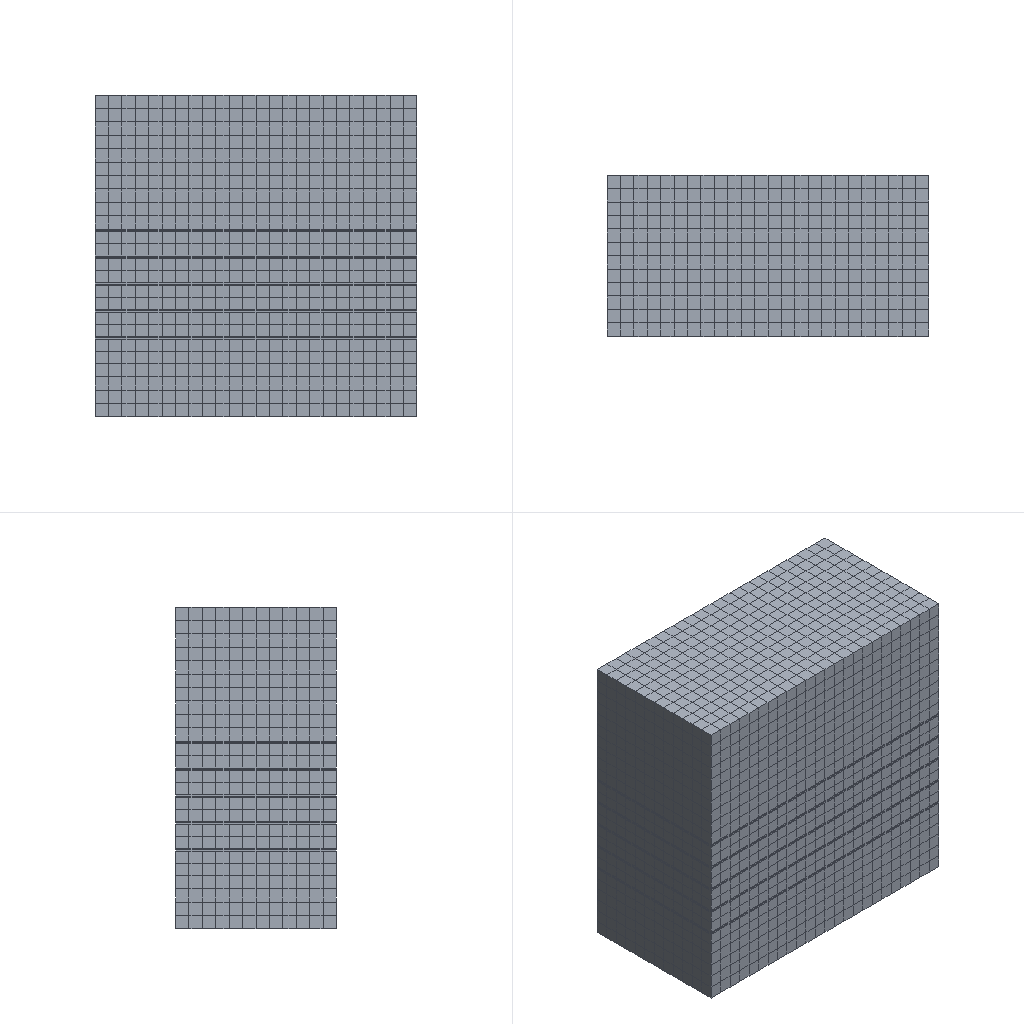Simulation study | abaqus
Set-up summary:
category,name,step,type,value,unit,region
solver,abaqus
solver,version,,,Abaqus/Standard 2020
units,not stated in the deck,,not stated
analysis,deck,,transient,transient
load_step,Step-1,Step-1,transient
load_step,requested,,,1
mesh,nodes,,,11845
mesh,elements,,,10259
element_type,R3D4,,rigid,467
element_type,C3D8R,,solid,9792
load,load commands in deck,,count,1
bc,support commands in deck,,count,7
material,CR,,in results
material,CRN,,in results
material,DLC,,in results
material,YG6,,in results
check,setup vs results,,match,"per instance, exact: element labels, types and connectivity; labels of the nodes the elements use; coordinates of those nodes at SINGLE_PRECISION in 2 of 2 instance(s)"
Abaqus input file, long lists of numbers shortened:
*Heading
** Job name: Job-1 Model name: Model-1
** Generated by: Abaqus/CAE 2020
*Preprint, echo=NO, model=NO, history=NO, contact=NO
**
** PARTS
**
*Part, name=work
*Node
      1, 0.0012,           0., 0.0002
      2, 0.0012, -0.0006, 0.0002
** (11373 more lines like these left out)
*Element, type=C3D8R
   1,  154, 1229, 5810, 1091,    1,   53, 1025,   80
   2, 1229, 1230, 5811, 5810,   53,   54, 1026, 1025
** (9790 more lines like these left out)
*Nset, nset=Set-1
    45,    46,    47,    48,    49,    50,    51,    52,   850,   851,   852,   853,   854,   855,   856,   857
   858,   859,   860,   863,   864,   865,   866,   867,   868,   869,   870,   871,   872,   873,   875,   876
** (222 more lines like these left out)
*Elset, elset=Set-1, generate
 6913,  9792,     1
*Nset, nset=Set-2
   41,   42,   43,   44,   45,   46,   47,   48,  778,  779,  780,  781,  782,  783,  784,  785
  786,  787,  788,  791,  792,  793,  794,  795,  796,  797,  798,  799,  800,  801,  803,  804
** (59 more lines like these left out)
*Elset, elset=Set-2, generate
 6337,  6912,     1
*Nset, nset=Set-3
   33,   34,   35,   36,   37,   38,   39,   40,  634,  635,  636,  637,  638,  639,  640,  641
  642,  643,  644,  647,  648,  649,  650,  651,  652,  653,  654,  655,  656,  657,  659,  660
** (59 more lines like these left out)
*Elset, elset=Set-3, generate
 5185,  5760,     1
*Nset, nset=Set-4
   25,   26,   27,   28,   29,   30,   31,   32,  490,  491,  492,  493,  494,  495,  496,  497
  498,  499,  500,  503,  504,  505,  506,  507,  508,  509,  510,  511,  512,  513,  515,  516
** (59 more lines like these left out)
*Elset, elset=Set-4, generate
 4033,  4608,     1
*Nset, nset=Set-5
   37,   38,   39,   40,   41,   42,   43,   44,  705,  706,  707,  708,  709,  710,  711,  712
  713,  714,  715,  718,  719,  720,  721,  722,  723,  724,  725,  726,  727,  728,  731,  732
** (59 more lines like these left out)
*Elset, elset=Set-5, generate
 5761,  6336,     1
*Nset, nset=Set-6
   21,   22,   23,   24,   25,   26,   27,   28,   29,   30,   31,   32,   33,   34,   35,   36
  417,  418,  419,  420,  421,  422,  423,  424,  425,  426,  427,  430,  431,  432,  433,  434
** (120 more lines like these left out)
*Elset, elset=Set-6
 3457, 3458, 3459, 3460, 3461, 3462, 3463, 3464, 3465, 3466, 3467, 3468, 3469, 3470, 3471, 3472
 3473, 3474, 3475, 3476, 3477, 3478, 3479, 3480, 3481, 3482, 3483, 3484, 3485, 3486, 3487, 3488
** (70 more lines like these left out)
*Nset, nset=Set-9
    9,   10,   11,   12,   13,   14,   15,   16,   17,   18,   19,   20,   21,   22,   23,   24
  202,  203,  204,  205,  206,  207,  208,  209,  210,  211,  212,  215,  216,  217,  218,  219
** (120 more lines like these left out)
*Elset, elset=Set-9
 1729, 1730, 1731, 1732, 1733, 1734, 1735, 1736, 1737, 1738, 1739, 1740, 1741, 1742, 1743, 1744
 1745, 1746, 1747, 1748, 1749, 1750, 1751, 1752, 1753, 1754, 1755, 1756, 1757, 1758, 1759, 1760
** (70 more lines like these left out)
*Nset, nset=Set-10
    1,    2,    5,    8,    9,   10,   11,   12,   13,   14,   15,   16,   17,   18,   19,   20
   53,   54,   55,   56,   57,   58,   59,   60,   61,   62,   63,   81,   82,   83,   84,   85
** (120 more lines like these left out)
*Elset, elset=Set-10
 1153, 1154, 1155, 1156, 1157, 1158, 1159, 1160, 1161, 1162, 1163, 1164, 1165, 1166, 1167, 1168
 1169, 1170, 1171, 1172, 1173, 1174, 1175, 1176, 1177, 1178, 1179, 1180, 1181, 1182, 1183, 1184
** (70 more lines like these left out)
*Nset, nset=Set-11
    1,    2,    3,    4,    5,    6,    7,    8,   53,   54,   55,   56,   57,   58,   59,   60
   61,   62,   63,   64,   65,   66,   67,   68,   69,   70,   71,   72,   73,   74,   75,   76
** (100 more lines like these left out)
*Elset, elset=Set-11, generate
    1,  1152,     1
** Section: yg6
*Solid Section, elset=Set-11, material=yg6
,
** Section: crN
*Solid Section, elset=Set-10, material=crN
,
** Section: cr
*Solid Section, elset=Set-9, material=cr
,
** Section: crN
*Solid Section, elset=Set-6, material=crN
,
** Section: cr
*Solid Section, elset=Set-4, material=cr
,
** Section: cr
*Solid Section, elset=Set-3, material=cr
,
** Section: crN
*Solid Section, elset=Set-5, material=crN
,
** Section: cr
*Solid Section, elset=Set-2, material=cr
,
** Section: dlc
*Solid Section, elset=Set-1, material=DLC
,
*End Part
**
*Part, name=zhui
*Node
      1, 0.0003, -0.0005196,           0.
      2,           0.,           0.,           0.
** (467 more lines like these left out)
*Element, type=R3D4
 1, 120,  95,  40,  41
 2,  39,  40,  95,  97
** (465 more lines like these left out)
*Node
    470, 5.29395592e-20, -0.0003464, 9.20947787e-05
*Nset, nset=zhui-RefPt_, internal
470,
*Elset, elset=zhui, generate
   1,  467,    1
*End Part
**
**
** ASSEMBLY
**
*Assembly, name=Assembly
**
*Instance, name=work-1, part=work
*End Instance
**
*Instance, name=zhui-1, part=zhui
      0.0006, -5.39999999999999e-05,     0.001292
      0.0006, -5.39999999999999e-05,     0.001292,       0.0006,     0.9999,     0.001292,         180.
*End Instance
**
*Nset, nset=Set-1, instance=work-1
    3,    4,    6,    7,   67,   68,   69,   70,   71,   72,   73,   74,   75,   76,   77,   95
   96,   97,   98,   99,  100,  101,  102,  103,  104,  105,  109,  110,  111,  112,  113,  114
** (19 more lines like these left out)
*Elset, elset=Set-1, instance=work-1
   37,   38,   39,   40,   41,   42,   43,   44,   45,   46,   47,   48,   85,   86,   87,   88
   89,   90,   91,   92,   93,   94,   95,   96,  133,  134,  135,  136,  137,  138,  139,  140
** (16 more lines like these left out)
*Nset, nset=Set-2, instance=zhui-1
 470,
*Elset, elset=_m_Surf-1_SPOS, internal, instance=zhui-1, generate
   1,  248,    1
*Surface, type=ELEMENT, name=m_Surf-1
_m_Surf-1_SPOS, SPOS
*Elset, elset=_s_Surf-1_S5, internal, instance=work-1
 7021, 7022, 7023, 7024, 7025, 7026, 7027, 7028, 7029, 7030, 7031, 7032, 7141, 7142, 7143, 7144
 7145, 7146, 7147, 7148, 7149, 7150, 7151, 7152, 7261, 7262, 7263, 7264, 7265, 7266, 7267, 7268
** (16 more lines like these left out)
*Surface, type=ELEMENT, name=s_Surf-1
_s_Surf-1_S5, S5
*Rigid Body, ref node=zhui-1.zhui-RefPt_, elset=zhui-1.zhui
*End Assembly
**
** MATERIALS
**
*Material, name=DLC
*Density
 4e-09,
*Elastic
258800., 0.3
*Material, name=cr
*Density
 7.19e-09,
*Elastic
275000., 0.21
*Plastic
2000.,  0.
5000., 0.1
5500.,  1.
*Material, name=crN
*Density
 5.9e-09,
*Elastic
490000., 0.21
*Plastic
10000.,   0.
15000., 0.01
25000., 0.05
*Material, name=yg6
*Density
 1.5e-08,
*Elastic
71000., 0.3
*Plastic
3000.,0.
**
** INTERACTION PROPERTIES
**
*Surface Interaction, name=IntProp-1
1.,
*Friction, slip tolerance=0.005
 0.3,
*Surface Behavior, pressure-overclosure=HARD
**
** BOUNDARY CONDITIONS
**
** Name: BC-1 Type: 对称/反对称/完全固定
*Boundary
Set-1, ENCASTRE
**
** INTERACTIONS
**
** Interaction: Int-1
*Contact Pair, interaction=IntProp-1, type=SURFACE TO SURFACE
s_Surf-1, m_Surf-1
** Interaction: Int-2
*Contact
*Contact Inclusions, ALL EXTERIOR
*Contact Property Assignment
 ,  , IntProp-1
** ----------------------------------------------------------------
**
** STEP: Step-1
**
*Step, name=Step-1, nlgeom=YES, inc=10000
*Dynamic
0.001,1.,1e-05
**
** BOUNDARY CONDITIONS
**
** Name: BC-2 Type: 位移/转角
*Boundary
Set-2, 1, 1
Set-2, 2, 2
Set-2, 3, 3, -0.0001
Set-2, 4, 4
Set-2, 5, 5
Set-2, 6, 6
**
** OUTPUT REQUESTS
**
*Restart, write, frequency=0
**
** FIELD OUTPUT: F-Output-1
**
*Output, field, frequency=1
*Node Output
A, CF, RF, U, V
*Element Output, directions=YES
E, LE, MISES, PE, PEEQ, PEMAG, S
*Contact Output
CDISP, CSTRESS
**
** HISTORY OUTPUT: H-Output-1
**
*Output, history, variable=PRESELECT
*End Step
Results summary:
result,step,,partial,increments=23 time=0.3083/1.0
result,analysis,,,transient
result,last_loadstep,,,1
result,primary field,,,U
result,reaction total,,FX,-0.0,model units
result,reaction total,,FY,0.000391,model units
result,reaction total,,FZ,8.3e-05,model units